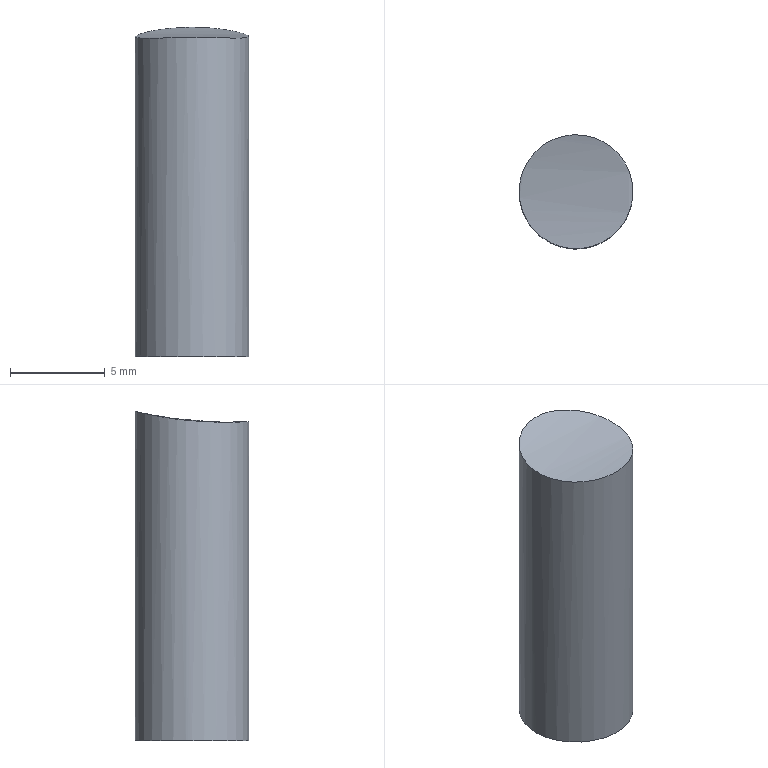Part | NX | features solid 2 | 1 solid | 3 faces | box 6 x 6 x 17.344 mm | volume 477.877 mm3 | cylinder 1 | plane 1 | spline 1 | commonest cylinder face diameters 6 x1
STEP:
#1=CARTESIAN_POINT('',(434.5,230.,25.));
#2=VERTEX_POINT('',#1);
#3=CARTESIAN_POINT('',(437.5,230.,25.));
#4=DIRECTION('',(0.,0.,-1.));
#5=DIRECTION('',(-1.,0.,0.));
#6=AXIS2_PLACEMENT_3D('',#3,#4,#5);
#7=CIRCLE('',#6,3.);
#8=EDGE_CURVE('',#2,#2,#7,.F.);
#9=ORIENTED_EDGE('',*,*,#8,.T.);
#10=EDGE_LOOP('',(#9));
#11=FACE_BOUND('',#10,.T.);
#12=CARTESIAN_POINT('',(434.518,230.33,41.877));
#13=VERTEX_POINT('',#12);
#14=CARTESIAN_POINT('',(435.411,232.583,42.225));
#15=CARTESIAN_POINT('',(434.198,230.37,41.824));
#16=CARTESIAN_POINT('',(434.906,227.916,41.74));
#17=CARTESIAN_POINT('',(437.145,226.693,41.827));
#18=CARTESIAN_POINT('',(439.597,227.415,41.775));
#19=CARTESIAN_POINT('',(440.807,229.668,41.77));
#20=CARTESIAN_POINT('',(440.083,232.086,42.114));
#21=CARTESIAN_POINT('',(437.857,233.307,42.427));
#22=CARTESIAN_POINT('',(435.411,232.583,42.225));
#23=CARTESIAN_POINT('',(434.198,230.37,41.824));
#24=CARTESIAN_POINT('',(434.906,227.916,41.74));
#25=B_SPLINE_CURVE_WITH_KNOTS('',3,(#14,#15,#16,#17,#18,#19,#20,#21,#22,#23,#24),.UNSPECIFIED.,.T.,.F.,(1,1,1,1,1,1,1,1,1,1,1,1,1,1,1),(-0.007058,-0.004705,-0.002353,0.,0.002353,0.004705,0.007058,0.009411,0.01176,0.01412,0.01647,0.01882,0.02117,0.02353,0.02588),.UNSPECIFIED.);
#26=EDGE_CURVE('',#13,#13,#25,.T.);
#27=ORIENTED_EDGE('',*,*,#26,.F.);
#28=EDGE_LOOP('',(#27));
#29=FACE_BOUND('',#28,.T.);
#30=CARTESIAN_POINT('',(437.5,230.,35.));
#31=DIRECTION('',(0.,0.,-1.));
#32=DIRECTION('',(1.,0.,0.));
#33=AXIS2_PLACEMENT_3D('',#30,#31,#32);
#34=CYLINDRICAL_SURFACE('',#33,3.);
#35=ADVANCED_FACE('',(#11,#29),#34,.T.);
#36=ORIENTED_EDGE('',*,*,#8,.F.);
#37=EDGE_LOOP('',(#36));
#38=FACE_BOUND('',#37,.T.);
#39=CARTESIAN_POINT('',(437.5,230.,25.));
#40=DIRECTION('',(0.,0.,-1.));
#41=DIRECTION('',(1.,0.,0.));
#42=AXIS2_PLACEMENT_3D('',#39,#40,#41);
#43=PLANE('',#42);
#44=ADVANCED_FACE('',(#38),#43,.T.);
#45=ORIENTED_EDGE('',*,*,#26,.T.);
#46=EDGE_LOOP('',(#45));
#47=FACE_BOUND('',#46,.T.);
#48=CARTESIAN_POINT('',(440.558,226.966,41.811));
#49=CARTESIAN_POINT('',(434.45,226.958,41.802));
#50=CARTESIAN_POINT('',(440.558,227.135,41.804));
#51=CARTESIAN_POINT('',(434.449,227.127,41.796));
#52=CARTESIAN_POINT('',(440.558,227.303,41.798));
#53=CARTESIAN_POINT('',(434.449,227.295,41.789));
#54=CARTESIAN_POINT('',(440.558,227.471,41.791));
#55=CARTESIAN_POINT('',(434.449,227.463,41.782));
#56=CARTESIAN_POINT('',(440.555,229.352,41.718));
#57=CARTESIAN_POINT('',(434.447,229.344,41.709));
#58=CARTESIAN_POINT('',(440.553,231.233,41.909));
#59=CARTESIAN_POINT('',(434.444,231.225,41.9));
#60=CARTESIAN_POINT('',(440.55,233.077,42.367));
#61=CARTESIAN_POINT('',(434.441,233.069,42.359));
#62=(BOUNDED_SURFACE()B_SPLINE_SURFACE(3,1,((#48,#49),(#50,#51),(#52,#53),(#54,#55),(#56,#57),(#58,#59),(#60,#61)),.SURF_OF_LINEAR_EXTRUSION.,.F.,.F.,.F.)B_SPLINE_SURFACE_WITH_KNOTS((4,3,4),(2,2),(-0.03914,0.,0.4309),(0.7915,0.8277),.PIECEWISE_BEZIER_KNOTS.)GEOMETRIC_REPRESENTATION_ITEM()RATIONAL_B_SPLINE_SURFACE(((1.,1.),(1.,1.),(1.,1.),(1.,1.),(0.9846,0.9846),(0.9759,0.9759),(0.9738,0.9738)))REPRESENTATION_ITEM('')SURFACE());
#63=ADVANCED_FACE('',(#47),#62,.T.);
#64=CLOSED_SHELL('',(#35,#44,#63));
#65=MANIFOLD_SOLID_BREP('',#64);
#66=(LENGTH_UNIT()NAMED_UNIT(*)SI_UNIT(.MILLI.,.METRE.));
#67=UNCERTAINTY_MEASURE_WITH_UNIT(LENGTH_MEASURE(0.0508),#66,'','');
#68=(NAMED_UNIT(*)PLANE_ANGLE_UNIT()SI_UNIT($,.RADIAN.));
#69=(NAMED_UNIT(*)SI_UNIT($,.STERADIAN.)SOLID_ANGLE_UNIT());
#70=(GEOMETRIC_REPRESENTATION_CONTEXT(3)GLOBAL_UNCERTAINTY_ASSIGNED_CONTEXT((#67))GLOBAL_UNIT_ASSIGNED_CONTEXT((#66,#68,#69))REPRESENTATION_CONTEXT('',''));
#71=ADVANCED_BREP_SHAPE_REPRESENTATION('',(#65),#70);